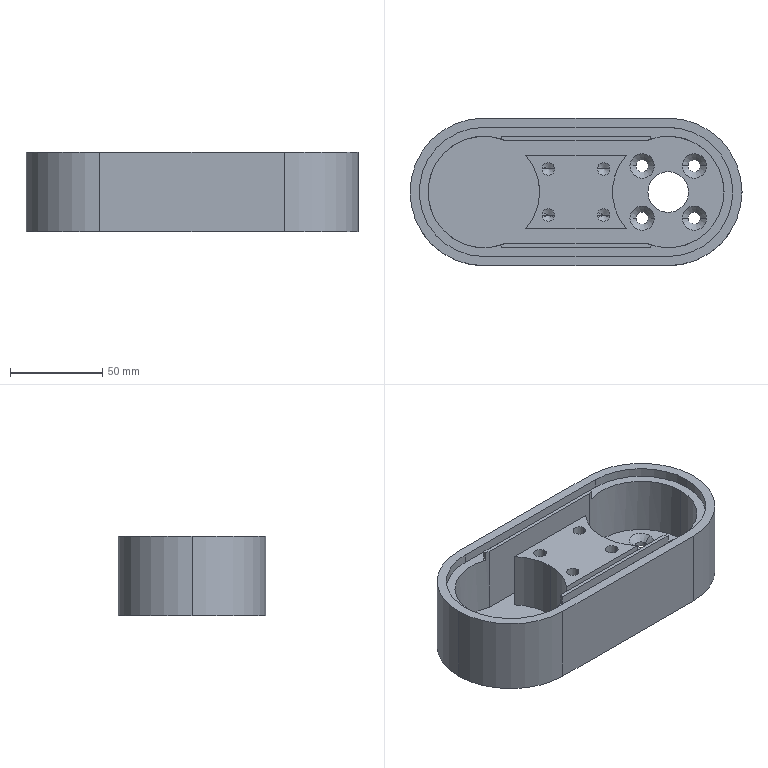Part | STEP file | Pulley box QY-1-09 | 1 solid | 67 faces | box 180 x 80 x 43 mm | volume 283710 mm3 | cylinder 30 | plane 21 | cone 16 | commonest cylinder face diameters 6.6 x8 6.8 x8 60.5 x6 70 x3 80 x3 22 x2